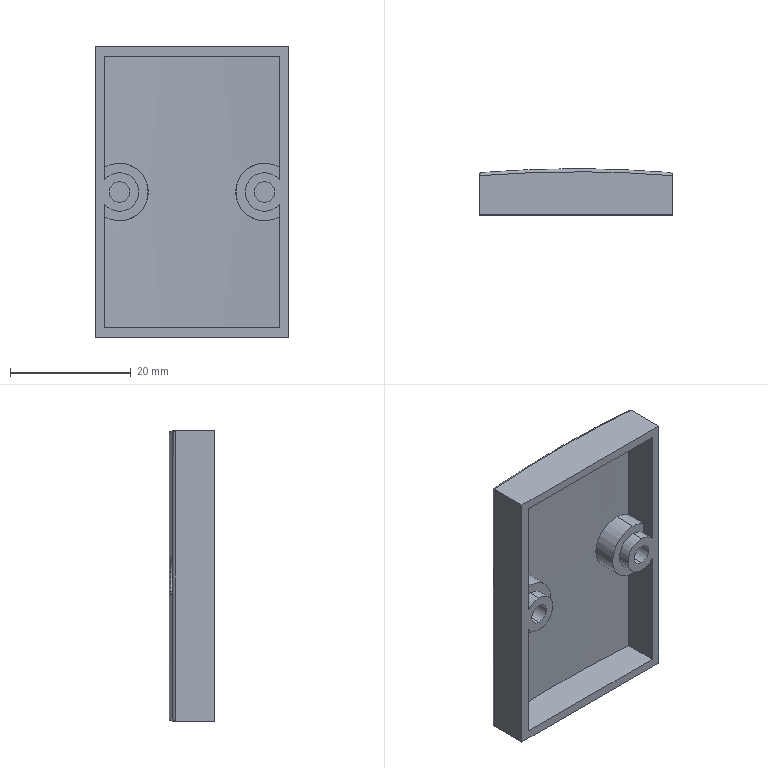Part | SolidWorks | features BaseBody 1 | 1 solid | 159 faces | box 32 x 7.6 x 48 mm | volume 3951 mm3 | plane 72 | spline 46 | cylinder 37 | cone 4 | commonest cylinder face diameters 399.2 x7 6.4 x6 9.5 x6 3.4 x4 5.5 x4 6.5 x4